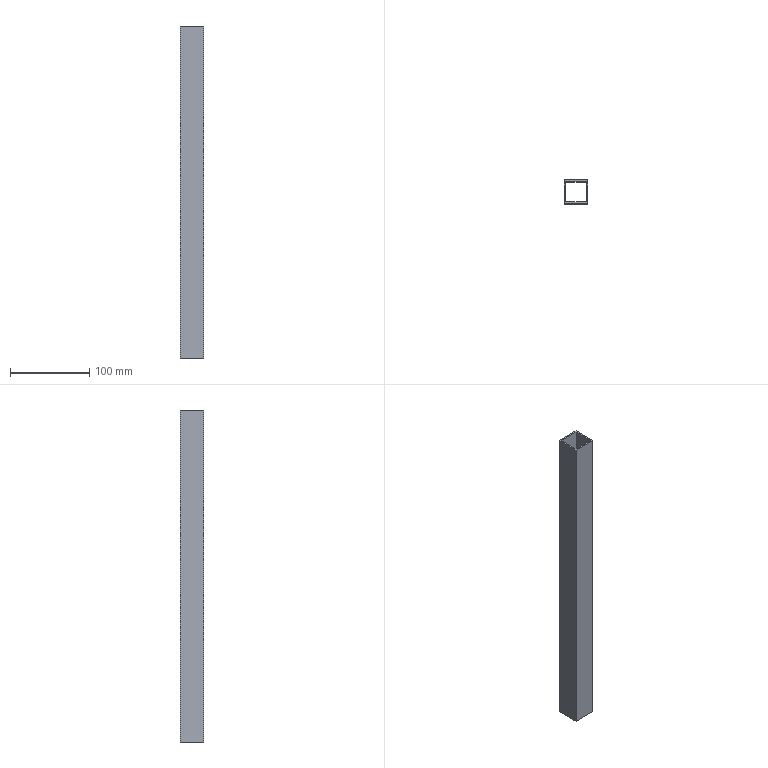Part | SolidWorks | features Extrusion 1 | 1 solid | 10 faces | box 30 x 30 x 420 mm | volume 94080 mm3 | plane 10
STEP:
#1=CARTESIAN_POINT('',(-15.,15.,210.));
#2=VERTEX_POINT('',#1);
#3=CARTESIAN_POINT('',(-15.,-15.,210.));
#4=VERTEX_POINT('',#3);
#5=CARTESIAN_POINT('',(-15.,-15.,210.));
#6=DIRECTION('',(0.,-1.,0.));
#7=VECTOR('',#6,1000.);
#8=LINE('',#5,#7);
#9=EDGE_CURVE('',#2,#4,#8,.T.);
#10=ORIENTED_EDGE('',*,*,#9,.T.);
#11=CARTESIAN_POINT('',(15.,-15.,210.));
#12=VERTEX_POINT('',#11);
#13=CARTESIAN_POINT('',(15.,-15.,210.));
#14=DIRECTION('',(1.,0.,0.));
#15=VECTOR('',#14,1000.);
#16=LINE('',#13,#15);
#17=EDGE_CURVE('',#4,#12,#16,.T.);
#18=ORIENTED_EDGE('',*,*,#17,.T.);
#19=CARTESIAN_POINT('',(15.,15.,210.));
#20=VERTEX_POINT('',#19);
#21=CARTESIAN_POINT('',(15.,-15.,210.));
#22=DIRECTION('',(0.,1.,0.));
#23=VECTOR('',#22,1000.);
#24=LINE('',#21,#23);
#25=EDGE_CURVE('',#12,#20,#24,.T.);
#26=ORIENTED_EDGE('',*,*,#25,.T.);
#27=CARTESIAN_POINT('',(15.,15.,210.));
#28=DIRECTION('',(-1.,0.,0.));
#29=VECTOR('',#28,1000.);
#30=LINE('',#27,#29);
#31=EDGE_CURVE('',#20,#2,#30,.T.);
#32=ORIENTED_EDGE('',*,*,#31,.T.);
#33=EDGE_LOOP('',(#10,#18,#26,#32));
#34=FACE_OUTER_BOUND('',#33,.T.);
#35=CARTESIAN_POINT('',(13.,13.,210.));
#36=VERTEX_POINT('',#35);
#37=CARTESIAN_POINT('',(-13.,13.,210.));
#38=VERTEX_POINT('',#37);
#39=CARTESIAN_POINT('',(13.,13.,210.));
#40=DIRECTION('',(-1.,0.,0.));
#41=VECTOR('',#40,1000.);
#42=LINE('',#39,#41);
#43=EDGE_CURVE('',#36,#38,#42,.T.);
#44=ORIENTED_EDGE('',*,*,#43,.F.);
#45=CARTESIAN_POINT('',(13.,-13.,210.));
#46=VERTEX_POINT('',#45);
#47=CARTESIAN_POINT('',(13.,-13.,210.));
#48=DIRECTION('',(0.,1.,0.));
#49=VECTOR('',#48,1000.);
#50=LINE('',#47,#49);
#51=EDGE_CURVE('',#46,#36,#50,.T.);
#52=ORIENTED_EDGE('',*,*,#51,.F.);
#53=CARTESIAN_POINT('',(-13.,-13.,210.));
#54=VERTEX_POINT('',#53);
#55=CARTESIAN_POINT('',(13.,-13.,210.));
#56=DIRECTION('',(1.,0.,0.));
#57=VECTOR('',#56,1000.);
#58=LINE('',#55,#57);
#59=EDGE_CURVE('',#54,#46,#58,.T.);
#60=ORIENTED_EDGE('',*,*,#59,.F.);
#61=CARTESIAN_POINT('',(-13.,-13.,210.));
#62=DIRECTION('',(0.,-1.,0.));
#63=VECTOR('',#62,1000.);
#64=LINE('',#61,#63);
#65=EDGE_CURVE('',#38,#54,#64,.T.);
#66=ORIENTED_EDGE('',*,*,#65,.F.);
#67=EDGE_LOOP('',(#44,#52,#60,#66));
#68=FACE_BOUND('',#67,.T.);
#69=CARTESIAN_POINT('',(0.,0.,210.));
#70=DIRECTION('',(0.,0.,1.));
#71=DIRECTION('',(1.,0.,0.));
#72=AXIS2_PLACEMENT_3D('',#69,#70,#71);
#73=PLANE('',#72);
#74=ADVANCED_FACE('',(#34,#68),#73,.T.);
#75=CARTESIAN_POINT('',(-15.,15.,-210.));
#76=VERTEX_POINT('',#75);
#77=CARTESIAN_POINT('',(-15.,-15.,-210.));
#78=VERTEX_POINT('',#77);
#79=CARTESIAN_POINT('',(-15.,-15.,-210.));
#80=DIRECTION('',(0.,-1.,0.));
#81=VECTOR('',#80,1000.);
#82=LINE('',#79,#81);
#83=EDGE_CURVE('',#76,#78,#82,.T.);
#84=ORIENTED_EDGE('',*,*,#83,.F.);
#85=CARTESIAN_POINT('',(15.,15.,-210.));
#86=VERTEX_POINT('',#85);
#87=CARTESIAN_POINT('',(15.,15.,-210.));
#88=DIRECTION('',(-1.,0.,0.));
#89=VECTOR('',#88,1000.);
#90=LINE('',#87,#89);
#91=EDGE_CURVE('',#86,#76,#90,.T.);
#92=ORIENTED_EDGE('',*,*,#91,.F.);
#93=CARTESIAN_POINT('',(15.,-15.,-210.));
#94=VERTEX_POINT('',#93);
#95=CARTESIAN_POINT('',(15.,-15.,-210.));
#96=DIRECTION('',(0.,1.,0.));
#97=VECTOR('',#96,1000.);
#98=LINE('',#95,#97);
#99=EDGE_CURVE('',#94,#86,#98,.T.);
#100=ORIENTED_EDGE('',*,*,#99,.F.);
#101=CARTESIAN_POINT('',(15.,-15.,-210.));
#102=DIRECTION('',(1.,0.,0.));
#103=VECTOR('',#102,1000.);
#104=LINE('',#101,#103);
#105=EDGE_CURVE('',#78,#94,#104,.T.);
#106=ORIENTED_EDGE('',*,*,#105,.F.);
#107=EDGE_LOOP('',(#84,#92,#100,#106));
#108=FACE_OUTER_BOUND('',#107,.T.);
#109=CARTESIAN_POINT('',(13.,-13.,-210.));
#110=VERTEX_POINT('',#109);
#111=CARTESIAN_POINT('',(13.,13.,-210.));
#112=VERTEX_POINT('',#111);
#113=CARTESIAN_POINT('',(13.,-13.,-210.));
#114=DIRECTION('',(0.,1.,0.));
#115=VECTOR('',#114,1000.);
#116=LINE('',#113,#115);
#117=EDGE_CURVE('',#110,#112,#116,.T.);
#118=ORIENTED_EDGE('',*,*,#117,.T.);
#119=CARTESIAN_POINT('',(-13.,13.,-210.));
#120=VERTEX_POINT('',#119);
#121=CARTESIAN_POINT('',(13.,13.,-210.));
#122=DIRECTION('',(-1.,0.,0.));
#123=VECTOR('',#122,1000.);
#124=LINE('',#121,#123);
#125=EDGE_CURVE('',#112,#120,#124,.T.);
#126=ORIENTED_EDGE('',*,*,#125,.T.);
#127=CARTESIAN_POINT('',(-13.,-13.,-210.));
#128=VERTEX_POINT('',#127);
#129=CARTESIAN_POINT('',(-13.,-13.,-210.));
#130=DIRECTION('',(0.,-1.,0.));
#131=VECTOR('',#130,1000.);
#132=LINE('',#129,#131);
#133=EDGE_CURVE('',#120,#128,#132,.T.);
#134=ORIENTED_EDGE('',*,*,#133,.T.);
#135=CARTESIAN_POINT('',(13.,-13.,-210.));
#136=DIRECTION('',(1.,0.,0.));
#137=VECTOR('',#136,1000.);
#138=LINE('',#135,#137);
#139=EDGE_CURVE('',#128,#110,#138,.T.);
#140=ORIENTED_EDGE('',*,*,#139,.T.);
#141=EDGE_LOOP('',(#118,#126,#134,#140));
#142=FACE_BOUND('',#141,.T.);
#143=CARTESIAN_POINT('',(0.,0.,-210.));
#144=DIRECTION('',(0.,0.,1.));
#145=DIRECTION('',(1.,0.,0.));
#146=AXIS2_PLACEMENT_3D('',#143,#144,#145);
#147=PLANE('',#146);
#148=ADVANCED_FACE('',(#108,#142),#147,.F.);
#149=ORIENTED_EDGE('',*,*,#83,.T.);
#150=CARTESIAN_POINT('',(-15.,-15.,210.));
#151=DIRECTION('',(0.,0.,-1.));
#152=VECTOR('',#151,1000.);
#153=LINE('',#150,#152);
#154=EDGE_CURVE('',#4,#78,#153,.T.);
#155=ORIENTED_EDGE('',*,*,#154,.F.);
#156=ORIENTED_EDGE('',*,*,#9,.F.);
#157=CARTESIAN_POINT('',(-15.,15.,210.));
#158=DIRECTION('',(0.,0.,-1.));
#159=VECTOR('',#158,1000.);
#160=LINE('',#157,#159);
#161=EDGE_CURVE('',#2,#76,#160,.T.);
#162=ORIENTED_EDGE('',*,*,#161,.T.);
#163=EDGE_LOOP('',(#149,#155,#156,#162));
#164=FACE_OUTER_BOUND('',#163,.T.);
#165=CARTESIAN_POINT('',(-15.,-15.,210.));
#166=DIRECTION('',(1.,0.,0.));
#167=DIRECTION('',(0.,1.,0.));
#168=AXIS2_PLACEMENT_3D('',#165,#166,#167);
#169=PLANE('',#168);
#170=ADVANCED_FACE('',(#164),#169,.F.);
#171=ORIENTED_EDGE('',*,*,#105,.T.);
#172=CARTESIAN_POINT('',(15.,-15.,210.));
#173=DIRECTION('',(0.,0.,-1.));
#174=VECTOR('',#173,1000.);
#175=LINE('',#172,#174);
#176=EDGE_CURVE('',#12,#94,#175,.T.);
#177=ORIENTED_EDGE('',*,*,#176,.F.);
#178=ORIENTED_EDGE('',*,*,#17,.F.);
#179=ORIENTED_EDGE('',*,*,#154,.T.);
#180=EDGE_LOOP('',(#171,#177,#178,#179));
#181=FACE_OUTER_BOUND('',#180,.T.);
#182=CARTESIAN_POINT('',(15.,-15.,210.));
#183=DIRECTION('',(0.,1.,0.));
#184=DIRECTION('',(-1.,0.,0.));
#185=AXIS2_PLACEMENT_3D('',#182,#183,#184);
#186=PLANE('',#185);
#187=ADVANCED_FACE('',(#181),#186,.F.);
#188=ORIENTED_EDGE('',*,*,#99,.T.);
#189=CARTESIAN_POINT('',(15.,15.,210.));
#190=DIRECTION('',(0.,0.,-1.));
#191=VECTOR('',#190,1000.);
#192=LINE('',#189,#191);
#193=EDGE_CURVE('',#20,#86,#192,.T.);
#194=ORIENTED_EDGE('',*,*,#193,.F.);
#195=ORIENTED_EDGE('',*,*,#25,.F.);
#196=ORIENTED_EDGE('',*,*,#176,.T.);
#197=EDGE_LOOP('',(#188,#194,#195,#196));
#198=FACE_OUTER_BOUND('',#197,.T.);
#199=CARTESIAN_POINT('',(15.,-15.,210.));
#200=DIRECTION('',(-1.,0.,0.));
#201=DIRECTION('',(0.,0.,1.));
#202=AXIS2_PLACEMENT_3D('',#199,#200,#201);
#203=PLANE('',#202);
#204=ADVANCED_FACE('',(#198),#203,.F.);
#205=ORIENTED_EDGE('',*,*,#91,.T.);
#206=ORIENTED_EDGE('',*,*,#161,.F.);
#207=ORIENTED_EDGE('',*,*,#31,.F.);
#208=ORIENTED_EDGE('',*,*,#193,.T.);
#209=EDGE_LOOP('',(#205,#206,#207,#208));
#210=FACE_OUTER_BOUND('',#209,.T.);
#211=CARTESIAN_POINT('',(15.,15.,210.));
#212=DIRECTION('',(0.,-1.,0.));
#213=DIRECTION('',(0.,0.,-1.));
#214=AXIS2_PLACEMENT_3D('',#211,#212,#213);
#215=PLANE('',#214);
#216=ADVANCED_FACE('',(#210),#215,.F.);
#217=ORIENTED_EDGE('',*,*,#117,.F.);
#218=CARTESIAN_POINT('',(13.,-13.,210.));
#219=DIRECTION('',(0.,0.,-1.));
#220=VECTOR('',#219,1000.);
#221=LINE('',#218,#220);
#222=EDGE_CURVE('',#46,#110,#221,.T.);
#223=ORIENTED_EDGE('',*,*,#222,.F.);
#224=ORIENTED_EDGE('',*,*,#51,.T.);
#225=CARTESIAN_POINT('',(13.,13.,210.));
#226=DIRECTION('',(0.,0.,-1.));
#227=VECTOR('',#226,1000.);
#228=LINE('',#225,#227);
#229=EDGE_CURVE('',#36,#112,#228,.T.);
#230=ORIENTED_EDGE('',*,*,#229,.T.);
#231=EDGE_LOOP('',(#217,#223,#224,#230));
#232=FACE_OUTER_BOUND('',#231,.T.);
#233=CARTESIAN_POINT('',(13.,-13.,210.));
#234=DIRECTION('',(-1.,0.,0.));
#235=DIRECTION('',(0.,0.,1.));
#236=AXIS2_PLACEMENT_3D('',#233,#234,#235);
#237=PLANE('',#236);
#238=ADVANCED_FACE('',(#232),#237,.T.);
#239=ORIENTED_EDGE('',*,*,#125,.F.);
#240=ORIENTED_EDGE('',*,*,#229,.F.);
#241=ORIENTED_EDGE('',*,*,#43,.T.);
#242=CARTESIAN_POINT('',(-13.,13.,210.));
#243=DIRECTION('',(0.,0.,-1.));
#244=VECTOR('',#243,1000.);
#245=LINE('',#242,#244);
#246=EDGE_CURVE('',#38,#120,#245,.T.);
#247=ORIENTED_EDGE('',*,*,#246,.T.);
#248=EDGE_LOOP('',(#239,#240,#241,#247));
#249=FACE_OUTER_BOUND('',#248,.T.);
#250=CARTESIAN_POINT('',(13.,13.,210.));
#251=DIRECTION('',(0.,-1.,0.));
#252=DIRECTION('',(0.,0.,-1.));
#253=AXIS2_PLACEMENT_3D('',#250,#251,#252);
#254=PLANE('',#253);
#255=ADVANCED_FACE('',(#249),#254,.T.);
#256=ORIENTED_EDGE('',*,*,#133,.F.);
#257=ORIENTED_EDGE('',*,*,#246,.F.);
#258=ORIENTED_EDGE('',*,*,#65,.T.);
#259=CARTESIAN_POINT('',(-13.,-13.,210.));
#260=DIRECTION('',(0.,0.,-1.));
#261=VECTOR('',#260,1000.);
#262=LINE('',#259,#261);
#263=EDGE_CURVE('',#54,#128,#262,.T.);
#264=ORIENTED_EDGE('',*,*,#263,.T.);
#265=EDGE_LOOP('',(#256,#257,#258,#264));
#266=FACE_OUTER_BOUND('',#265,.T.);
#267=CARTESIAN_POINT('',(-13.,-13.,210.));
#268=DIRECTION('',(1.,0.,0.));
#269=DIRECTION('',(0.,0.,-1.));
#270=AXIS2_PLACEMENT_3D('',#267,#268,#269);
#271=PLANE('',#270);
#272=ADVANCED_FACE('',(#266),#271,.T.);
#273=ORIENTED_EDGE('',*,*,#139,.F.);
#274=ORIENTED_EDGE('',*,*,#263,.F.);
#275=ORIENTED_EDGE('',*,*,#59,.T.);
#276=ORIENTED_EDGE('',*,*,#222,.T.);
#277=EDGE_LOOP('',(#273,#274,#275,#276));
#278=FACE_OUTER_BOUND('',#277,.T.);
#279=CARTESIAN_POINT('',(13.,-13.,210.));
#280=DIRECTION('',(0.,1.,0.));
#281=DIRECTION('',(0.,0.,1.));
#282=AXIS2_PLACEMENT_3D('',#279,#280,#281);
#283=PLANE('',#282);
#284=ADVANCED_FACE('',(#278),#283,.T.);
#285=CLOSED_SHELL('',(#74,#148,#170,#187,#204,#216,#238,#255,#272,#284));
#286=MANIFOLD_SOLID_BREP('',#285);
#287=CARTESIAN_POINT('',(0.,0.,0.));
#288=DIRECTION('',(0.,0.,1.));
#289=DIRECTION('',(1.,0.,0.));
#290=AXIS2_PLACEMENT_3D('',#287,#288,#289);
#291=(LENGTH_UNIT()NAMED_UNIT(*)SI_UNIT(.MILLI.,.METRE.));
#292=UNCERTAINTY_MEASURE_WITH_UNIT(LENGTH_MEASURE(0.00001),#291,'','');
#293=(NAMED_UNIT(*)PLANE_ANGLE_UNIT()SI_UNIT($,.RADIAN.));
#294=(NAMED_UNIT(*)SI_UNIT($,.STERADIAN.)SOLID_ANGLE_UNIT());
#295=(GEOMETRIC_REPRESENTATION_CONTEXT(3)GLOBAL_UNCERTAINTY_ASSIGNED_CONTEXT((#292))GLOBAL_UNIT_ASSIGNED_CONTEXT((#291,#293,#294))REPRESENTATION_CONTEXT('',''));
#296=ADVANCED_BREP_SHAPE_REPRESENTATION('',(#286,#290),#295);